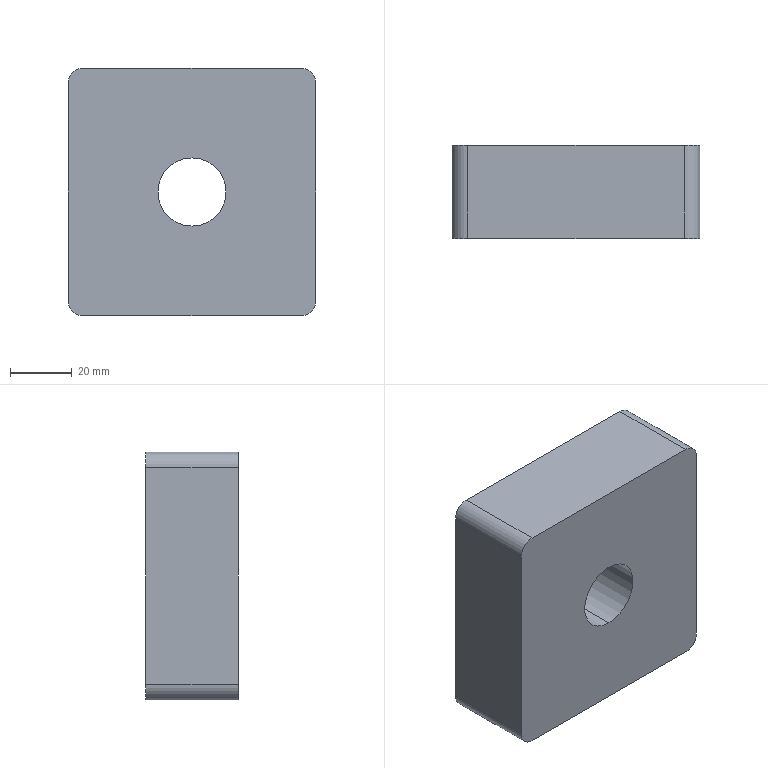Part | SolidWorks | features Extrusion 1, Fillet 1, HoleWzd 1 | 1 solid | 12 faces | box 80 x 30 x 80 mm | volume 179952 mm3 | cylinder 6 | plane 6 | commonest cylinder face diameters 10 x4 22 x2
STEP:
#1=CARTESIAN_POINT('',(0.,0.,-11.));
#2=VERTEX_POINT('',#1);
#3=CARTESIAN_POINT('',(0.,0.,11.));
#4=VERTEX_POINT('',#3);
#5=CARTESIAN_POINT('',(0.,0.,0.));
#6=DIRECTION('',(0.,1.,0.));
#7=DIRECTION('',(0.,0.,1.));
#8=AXIS2_PLACEMENT_3D('',#5,#6,#7);
#9=CIRCLE('',#8,11.);
#10=EDGE_CURVE('',#2,#4,#9,.T.);
#11=ORIENTED_EDGE('',*,*,#10,.F.);
#12=CARTESIAN_POINT('',(0.,30.,-11.));
#13=VERTEX_POINT('',#12);
#14=CARTESIAN_POINT('',(0.,30.,-11.));
#15=DIRECTION('',(0.,1.,0.));
#16=VECTOR('',#15,1000.);
#17=LINE('',#14,#16);
#18=EDGE_CURVE('',#2,#13,#17,.T.);
#19=ORIENTED_EDGE('',*,*,#18,.T.);
#20=CARTESIAN_POINT('',(0.,30.,11.));
#21=VERTEX_POINT('',#20);
#22=CARTESIAN_POINT('',(0.,30.,0.));
#23=DIRECTION('',(0.,1.,0.));
#24=DIRECTION('',(0.,0.,1.));
#25=AXIS2_PLACEMENT_3D('',#22,#23,#24);
#26=CIRCLE('',#25,11.);
#27=EDGE_CURVE('',#13,#21,#26,.T.);
#28=ORIENTED_EDGE('',*,*,#27,.T.);
#29=CARTESIAN_POINT('',(0.,30.,11.));
#30=DIRECTION('',(0.,1.,0.));
#31=VECTOR('',#30,1000.);
#32=LINE('',#29,#31);
#33=EDGE_CURVE('',#4,#21,#32,.T.);
#34=ORIENTED_EDGE('',*,*,#33,.F.);
#35=EDGE_LOOP('',(#11,#19,#28,#34));
#36=FACE_OUTER_BOUND('',#35,.T.);
#37=CARTESIAN_POINT('',(0.,30.,0.));
#38=DIRECTION('',(0.,1.,0.));
#39=DIRECTION('',(0.,0.,1.));
#40=AXIS2_PLACEMENT_3D('',#37,#38,#39);
#41=CYLINDRICAL_SURFACE('',#40,11.);
#42=ADVANCED_FACE('',(#36),#41,.F.);
#43=CARTESIAN_POINT('',(40.,0.,35.));
#44=VERTEX_POINT('',#43);
#45=CARTESIAN_POINT('',(40.,0.,-35.));
#46=VERTEX_POINT('',#45);
#47=CARTESIAN_POINT('',(40.,0.,-40.));
#48=DIRECTION('',(0.,0.,-1.));
#49=VECTOR('',#48,1000.);
#50=LINE('',#47,#49);
#51=EDGE_CURVE('',#44,#46,#50,.T.);
#52=ORIENTED_EDGE('',*,*,#51,.T.);
#53=CARTESIAN_POINT('',(40.,30.,-35.));
#54=VERTEX_POINT('',#53);
#55=CARTESIAN_POINT('',(40.,30.,-35.));
#56=DIRECTION('',(0.,1.,0.));
#57=VECTOR('',#56,1000.);
#58=LINE('',#55,#57);
#59=EDGE_CURVE('',#46,#54,#58,.T.);
#60=ORIENTED_EDGE('',*,*,#59,.T.);
#61=CARTESIAN_POINT('',(40.,30.,35.));
#62=VERTEX_POINT('',#61);
#63=CARTESIAN_POINT('',(40.,30.,-40.));
#64=DIRECTION('',(0.,0.,-1.));
#65=VECTOR('',#64,1000.);
#66=LINE('',#63,#65);
#67=EDGE_CURVE('',#62,#54,#66,.T.);
#68=ORIENTED_EDGE('',*,*,#67,.F.);
#69=CARTESIAN_POINT('',(40.,30.,35.));
#70=DIRECTION('',(0.,-1.,0.));
#71=VECTOR('',#70,1000.);
#72=LINE('',#69,#71);
#73=EDGE_CURVE('',#62,#44,#72,.T.);
#74=ORIENTED_EDGE('',*,*,#73,.T.);
#75=EDGE_LOOP('',(#52,#60,#68,#74));
#76=FACE_OUTER_BOUND('',#75,.T.);
#77=CARTESIAN_POINT('',(40.,30.,-40.));
#78=DIRECTION('',(-1.,0.,0.));
#79=DIRECTION('',(0.,0.,1.));
#80=AXIS2_PLACEMENT_3D('',#77,#78,#79);
#81=PLANE('',#80);
#82=ADVANCED_FACE('',(#76),#81,.F.);
#83=CARTESIAN_POINT('',(35.,0.,-40.));
#84=VERTEX_POINT('',#83);
#85=CARTESIAN_POINT('',(-35.,0.,-40.));
#86=VERTEX_POINT('',#85);
#87=CARTESIAN_POINT('',(-40.,0.,-40.));
#88=DIRECTION('',(-1.,0.,0.));
#89=VECTOR('',#88,1000.);
#90=LINE('',#87,#89);
#91=EDGE_CURVE('',#84,#86,#90,.T.);
#92=ORIENTED_EDGE('',*,*,#91,.T.);
#93=CARTESIAN_POINT('',(-35.,30.,-40.));
#94=VERTEX_POINT('',#93);
#95=CARTESIAN_POINT('',(-35.,30.,-40.));
#96=DIRECTION('',(0.,1.,0.));
#97=VECTOR('',#96,1000.);
#98=LINE('',#95,#97);
#99=EDGE_CURVE('',#86,#94,#98,.T.);
#100=ORIENTED_EDGE('',*,*,#99,.T.);
#101=CARTESIAN_POINT('',(35.,30.,-40.));
#102=VERTEX_POINT('',#101);
#103=CARTESIAN_POINT('',(-40.,30.,-40.));
#104=DIRECTION('',(-1.,0.,0.));
#105=VECTOR('',#104,1000.);
#106=LINE('',#103,#105);
#107=EDGE_CURVE('',#102,#94,#106,.T.);
#108=ORIENTED_EDGE('',*,*,#107,.F.);
#109=CARTESIAN_POINT('',(35.,30.,-40.));
#110=DIRECTION('',(0.,-1.,0.));
#111=VECTOR('',#110,1000.);
#112=LINE('',#109,#111);
#113=EDGE_CURVE('',#102,#84,#112,.T.);
#114=ORIENTED_EDGE('',*,*,#113,.T.);
#115=EDGE_LOOP('',(#92,#100,#108,#114));
#116=FACE_OUTER_BOUND('',#115,.T.);
#117=CARTESIAN_POINT('',(-40.,30.,-40.));
#118=DIRECTION('',(0.,0.,1.));
#119=DIRECTION('',(1.,0.,0.));
#120=AXIS2_PLACEMENT_3D('',#117,#118,#119);
#121=PLANE('',#120);
#122=ADVANCED_FACE('',(#116),#121,.F.);
#123=CARTESIAN_POINT('',(-40.,30.,-35.));
#124=VERTEX_POINT('',#123);
#125=CARTESIAN_POINT('',(-40.,30.,35.));
#126=VERTEX_POINT('',#125);
#127=CARTESIAN_POINT('',(-40.,30.,-40.));
#128=DIRECTION('',(0.,0.,1.));
#129=VECTOR('',#128,1000.);
#130=LINE('',#127,#129);
#131=EDGE_CURVE('',#124,#126,#130,.T.);
#132=ORIENTED_EDGE('',*,*,#131,.F.);
#133=CARTESIAN_POINT('',(-40.,0.,-35.));
#134=VERTEX_POINT('',#133);
#135=CARTESIAN_POINT('',(-40.,30.,-35.));
#136=DIRECTION('',(0.,-1.,0.));
#137=VECTOR('',#136,1000.);
#138=LINE('',#135,#137);
#139=EDGE_CURVE('',#124,#134,#138,.T.);
#140=ORIENTED_EDGE('',*,*,#139,.T.);
#141=CARTESIAN_POINT('',(-40.,0.,35.));
#142=VERTEX_POINT('',#141);
#143=CARTESIAN_POINT('',(-40.,0.,-40.));
#144=DIRECTION('',(0.,0.,1.));
#145=VECTOR('',#144,1000.);
#146=LINE('',#143,#145);
#147=EDGE_CURVE('',#134,#142,#146,.T.);
#148=ORIENTED_EDGE('',*,*,#147,.T.);
#149=CARTESIAN_POINT('',(-40.,30.,35.));
#150=DIRECTION('',(0.,1.,0.));
#151=VECTOR('',#150,1000.);
#152=LINE('',#149,#151);
#153=EDGE_CURVE('',#142,#126,#152,.T.);
#154=ORIENTED_EDGE('',*,*,#153,.T.);
#155=EDGE_LOOP('',(#132,#140,#148,#154));
#156=FACE_OUTER_BOUND('',#155,.T.);
#157=CARTESIAN_POINT('',(-40.,30.,-40.));
#158=DIRECTION('',(1.,0.,0.));
#159=DIRECTION('',(0.,0.,-1.));
#160=AXIS2_PLACEMENT_3D('',#157,#158,#159);
#161=PLANE('',#160);
#162=ADVANCED_FACE('',(#156),#161,.F.);
#163=CARTESIAN_POINT('',(-35.,0.,40.));
#164=VERTEX_POINT('',#163);
#165=CARTESIAN_POINT('',(35.,0.,40.));
#166=VERTEX_POINT('',#165);
#167=CARTESIAN_POINT('',(-40.,0.,40.));
#168=DIRECTION('',(1.,0.,0.));
#169=VECTOR('',#168,1000.);
#170=LINE('',#167,#169);
#171=EDGE_CURVE('',#164,#166,#170,.T.);
#172=ORIENTED_EDGE('',*,*,#171,.T.);
#173=CARTESIAN_POINT('',(35.,30.,40.));
#174=VERTEX_POINT('',#173);
#175=CARTESIAN_POINT('',(35.,30.,40.));
#176=DIRECTION('',(0.,1.,0.));
#177=VECTOR('',#176,1000.);
#178=LINE('',#175,#177);
#179=EDGE_CURVE('',#166,#174,#178,.T.);
#180=ORIENTED_EDGE('',*,*,#179,.T.);
#181=CARTESIAN_POINT('',(-35.,30.,40.));
#182=VERTEX_POINT('',#181);
#183=CARTESIAN_POINT('',(-40.,30.,40.));
#184=DIRECTION('',(1.,0.,0.));
#185=VECTOR('',#184,1000.);
#186=LINE('',#183,#185);
#187=EDGE_CURVE('',#182,#174,#186,.T.);
#188=ORIENTED_EDGE('',*,*,#187,.F.);
#189=CARTESIAN_POINT('',(-35.,30.,40.));
#190=DIRECTION('',(0.,-1.,0.));
#191=VECTOR('',#190,1000.);
#192=LINE('',#189,#191);
#193=EDGE_CURVE('',#182,#164,#192,.T.);
#194=ORIENTED_EDGE('',*,*,#193,.T.);
#195=EDGE_LOOP('',(#172,#180,#188,#194));
#196=FACE_OUTER_BOUND('',#195,.T.);
#197=CARTESIAN_POINT('',(-40.,30.,40.));
#198=DIRECTION('',(0.,0.,-1.));
#199=DIRECTION('',(-1.,0.,0.));
#200=AXIS2_PLACEMENT_3D('',#197,#198,#199);
#201=PLANE('',#200);
#202=ADVANCED_FACE('',(#196),#201,.F.);
#203=CARTESIAN_POINT('',(0.,30.,0.));
#204=DIRECTION('',(0.,1.,0.));
#205=DIRECTION('',(0.,0.,1.));
#206=AXIS2_PLACEMENT_3D('',#203,#204,#205);
#207=CIRCLE('',#206,11.);
#208=EDGE_CURVE('',#21,#13,#207,.T.);
#209=ORIENTED_EDGE('',*,*,#208,.F.);
#210=ORIENTED_EDGE('',*,*,#27,.F.);
#211=EDGE_LOOP('',(#209,#210));
#212=FACE_BOUND('',#211,.T.);
#213=ORIENTED_EDGE('',*,*,#107,.T.);
#214=CARTESIAN_POINT('',(-35.,30.,-35.));
#215=DIRECTION('',(0.,1.,0.));
#216=DIRECTION('',(0.,0.,1.));
#217=AXIS2_PLACEMENT_3D('',#214,#215,#216);
#218=CIRCLE('',#217,5.);
#219=EDGE_CURVE('',#94,#124,#218,.T.);
#220=ORIENTED_EDGE('',*,*,#219,.T.);
#221=ORIENTED_EDGE('',*,*,#131,.T.);
#222=CARTESIAN_POINT('',(-35.,30.,35.));
#223=DIRECTION('',(0.,1.,0.));
#224=DIRECTION('',(0.,0.,1.));
#225=AXIS2_PLACEMENT_3D('',#222,#223,#224);
#226=CIRCLE('',#225,5.);
#227=EDGE_CURVE('',#126,#182,#226,.T.);
#228=ORIENTED_EDGE('',*,*,#227,.T.);
#229=ORIENTED_EDGE('',*,*,#187,.T.);
#230=CARTESIAN_POINT('',(35.,30.,35.));
#231=DIRECTION('',(0.,1.,0.));
#232=DIRECTION('',(0.,0.,1.));
#233=AXIS2_PLACEMENT_3D('',#230,#231,#232);
#234=CIRCLE('',#233,5.);
#235=EDGE_CURVE('',#174,#62,#234,.T.);
#236=ORIENTED_EDGE('',*,*,#235,.T.);
#237=ORIENTED_EDGE('',*,*,#67,.T.);
#238=CARTESIAN_POINT('',(35.,30.,-35.));
#239=DIRECTION('',(0.,1.,0.));
#240=DIRECTION('',(0.,0.,1.));
#241=AXIS2_PLACEMENT_3D('',#238,#239,#240);
#242=CIRCLE('',#241,5.);
#243=EDGE_CURVE('',#54,#102,#242,.T.);
#244=ORIENTED_EDGE('',*,*,#243,.T.);
#245=EDGE_LOOP('',(#213,#220,#221,#228,#229,#236,#237,#244));
#246=FACE_OUTER_BOUND('',#245,.T.);
#247=CARTESIAN_POINT('',(0.,30.,0.));
#248=DIRECTION('',(0.,1.,0.));
#249=DIRECTION('',(0.,0.,1.));
#250=AXIS2_PLACEMENT_3D('',#247,#248,#249);
#251=PLANE('',#250);
#252=ADVANCED_FACE('',(#212,#246),#251,.T.);
#253=CARTESIAN_POINT('',(0.,0.,0.));
#254=DIRECTION('',(0.,1.,0.));
#255=DIRECTION('',(0.,0.,1.));
#256=AXIS2_PLACEMENT_3D('',#253,#254,#255);
#257=CIRCLE('',#256,11.);
#258=EDGE_CURVE('',#4,#2,#257,.T.);
#259=ORIENTED_EDGE('',*,*,#258,.T.);
#260=ORIENTED_EDGE('',*,*,#10,.T.);
#261=EDGE_LOOP('',(#259,#260));
#262=FACE_BOUND('',#261,.T.);
#263=ORIENTED_EDGE('',*,*,#147,.F.);
#264=CARTESIAN_POINT('',(-35.,0.,-35.));
#265=DIRECTION('',(0.,-1.,0.));
#266=DIRECTION('',(0.,0.,1.));
#267=AXIS2_PLACEMENT_3D('',#264,#265,#266);
#268=CIRCLE('',#267,5.);
#269=EDGE_CURVE('',#134,#86,#268,.T.);
#270=ORIENTED_EDGE('',*,*,#269,.T.);
#271=ORIENTED_EDGE('',*,*,#91,.F.);
#272=CARTESIAN_POINT('',(35.,0.,-35.));
#273=DIRECTION('',(0.,-1.,0.));
#274=DIRECTION('',(0.,0.,1.));
#275=AXIS2_PLACEMENT_3D('',#272,#273,#274);
#276=CIRCLE('',#275,5.);
#277=EDGE_CURVE('',#84,#46,#276,.T.);
#278=ORIENTED_EDGE('',*,*,#277,.T.);
#279=ORIENTED_EDGE('',*,*,#51,.F.);
#280=CARTESIAN_POINT('',(35.,0.,35.));
#281=DIRECTION('',(0.,-1.,0.));
#282=DIRECTION('',(0.,0.,1.));
#283=AXIS2_PLACEMENT_3D('',#280,#281,#282);
#284=CIRCLE('',#283,5.);
#285=EDGE_CURVE('',#44,#166,#284,.T.);
#286=ORIENTED_EDGE('',*,*,#285,.T.);
#287=ORIENTED_EDGE('',*,*,#171,.F.);
#288=CARTESIAN_POINT('',(-35.,0.,35.));
#289=DIRECTION('',(0.,-1.,0.));
#290=DIRECTION('',(0.,0.,1.));
#291=AXIS2_PLACEMENT_3D('',#288,#289,#290);
#292=CIRCLE('',#291,5.);
#293=EDGE_CURVE('',#164,#142,#292,.T.);
#294=ORIENTED_EDGE('',*,*,#293,.T.);
#295=EDGE_LOOP('',(#263,#270,#271,#278,#279,#286,#287,#294));
#296=FACE_OUTER_BOUND('',#295,.T.);
#297=CARTESIAN_POINT('',(0.,0.,0.));
#298=DIRECTION('',(0.,1.,0.));
#299=DIRECTION('',(0.,0.,1.));
#300=AXIS2_PLACEMENT_3D('',#297,#298,#299);
#301=PLANE('',#300);
#302=ADVANCED_FACE('',(#262,#296),#301,.F.);
#303=ORIENTED_EDGE('',*,*,#219,.F.);
#304=ORIENTED_EDGE('',*,*,#99,.F.);
#305=ORIENTED_EDGE('',*,*,#269,.F.);
#306=ORIENTED_EDGE('',*,*,#139,.F.);
#307=EDGE_LOOP('',(#303,#304,#305,#306));
#308=FACE_OUTER_BOUND('',#307,.T.);
#309=CARTESIAN_POINT('',(-35.,30.,-35.));
#310=DIRECTION('',(0.,-1.,0.));
#311=DIRECTION('',(0.,0.,-1.));
#312=AXIS2_PLACEMENT_3D('',#309,#310,#311);
#313=CYLINDRICAL_SURFACE('',#312,5.);
#314=ADVANCED_FACE('',(#308),#313,.T.);
#315=ORIENTED_EDGE('',*,*,#243,.F.);
#316=ORIENTED_EDGE('',*,*,#59,.F.);
#317=ORIENTED_EDGE('',*,*,#277,.F.);
#318=ORIENTED_EDGE('',*,*,#113,.F.);
#319=EDGE_LOOP('',(#315,#316,#317,#318));
#320=FACE_OUTER_BOUND('',#319,.T.);
#321=CARTESIAN_POINT('',(35.,30.,-35.));
#322=DIRECTION('',(0.,-1.,0.));
#323=DIRECTION('',(0.,0.,-1.));
#324=AXIS2_PLACEMENT_3D('',#321,#322,#323);
#325=CYLINDRICAL_SURFACE('',#324,5.);
#326=ADVANCED_FACE('',(#320),#325,.T.);
#327=ORIENTED_EDGE('',*,*,#235,.F.);
#328=ORIENTED_EDGE('',*,*,#179,.F.);
#329=ORIENTED_EDGE('',*,*,#285,.F.);
#330=ORIENTED_EDGE('',*,*,#73,.F.);
#331=EDGE_LOOP('',(#327,#328,#329,#330));
#332=FACE_OUTER_BOUND('',#331,.T.);
#333=CARTESIAN_POINT('',(35.,30.,35.));
#334=DIRECTION('',(0.,-1.,0.));
#335=DIRECTION('',(0.,0.,-1.));
#336=AXIS2_PLACEMENT_3D('',#333,#334,#335);
#337=CYLINDRICAL_SURFACE('',#336,5.);
#338=ADVANCED_FACE('',(#332),#337,.T.);
#339=ORIENTED_EDGE('',*,*,#227,.F.);
#340=ORIENTED_EDGE('',*,*,#153,.F.);
#341=ORIENTED_EDGE('',*,*,#293,.F.);
#342=ORIENTED_EDGE('',*,*,#193,.F.);
#343=EDGE_LOOP('',(#339,#340,#341,#342));
#344=FACE_OUTER_BOUND('',#343,.T.);
#345=CARTESIAN_POINT('',(-35.,30.,35.));
#346=DIRECTION('',(0.,-1.,0.));
#347=DIRECTION('',(0.,0.,-1.));
#348=AXIS2_PLACEMENT_3D('',#345,#346,#347);
#349=CYLINDRICAL_SURFACE('',#348,5.);
#350=ADVANCED_FACE('',(#344),#349,.T.);
#351=ORIENTED_EDGE('',*,*,#18,.F.);
#352=ORIENTED_EDGE('',*,*,#258,.F.);
#353=ORIENTED_EDGE('',*,*,#33,.T.);
#354=ORIENTED_EDGE('',*,*,#208,.T.);
#355=EDGE_LOOP('',(#351,#352,#353,#354));
#356=FACE_OUTER_BOUND('',#355,.T.);
#357=CARTESIAN_POINT('',(0.,30.,0.));
#358=DIRECTION('',(0.,1.,0.));
#359=DIRECTION('',(0.,0.,1.));
#360=AXIS2_PLACEMENT_3D('',#357,#358,#359);
#361=CYLINDRICAL_SURFACE('',#360,11.);
#362=ADVANCED_FACE('',(#356),#361,.F.);
#363=CLOSED_SHELL('',(#42,#82,#122,#162,#202,#252,#302,#314,#326,#338,#350,#362));
#364=MANIFOLD_SOLID_BREP('',#363);
#365=CARTESIAN_POINT('',(0.,0.,0.));
#366=DIRECTION('',(0.,0.,1.));
#367=DIRECTION('',(1.,0.,0.));
#368=AXIS2_PLACEMENT_3D('',#365,#366,#367);
#369=(LENGTH_UNIT()NAMED_UNIT(*)SI_UNIT(.MILLI.,.METRE.));
#370=UNCERTAINTY_MEASURE_WITH_UNIT(LENGTH_MEASURE(0.00001),#369,'','');
#371=(NAMED_UNIT(*)PLANE_ANGLE_UNIT()SI_UNIT($,.RADIAN.));
#372=(NAMED_UNIT(*)SI_UNIT($,.STERADIAN.)SOLID_ANGLE_UNIT());
#373=(GEOMETRIC_REPRESENTATION_CONTEXT(3)GLOBAL_UNCERTAINTY_ASSIGNED_CONTEXT((#370))GLOBAL_UNIT_ASSIGNED_CONTEXT((#369,#371,#372))REPRESENTATION_CONTEXT('',''));
#374=ADVANCED_BREP_SHAPE_REPRESENTATION('',(#364,#368),#373);